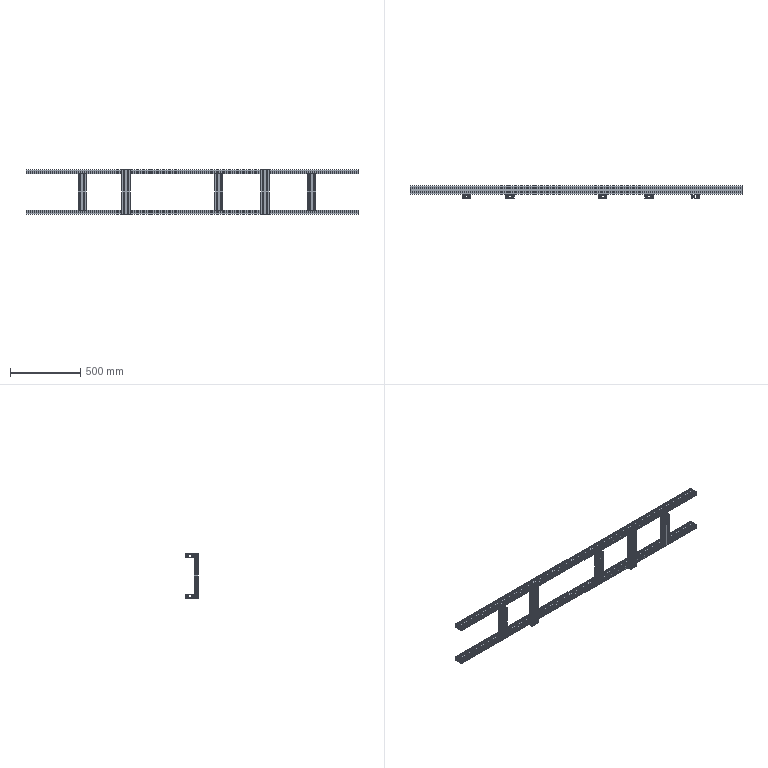Part | STEP file | welding conveyor bracket 01_Default <Machining> | 7 solids | 814 faces | box 2360 x 90 x 316 mm | volume 3445395 mm3 | plane 658 | cylinder 156 | commonest cylinder face diameters 4.2 x56 0.6 x28 2 x28 8 x28 12 x16